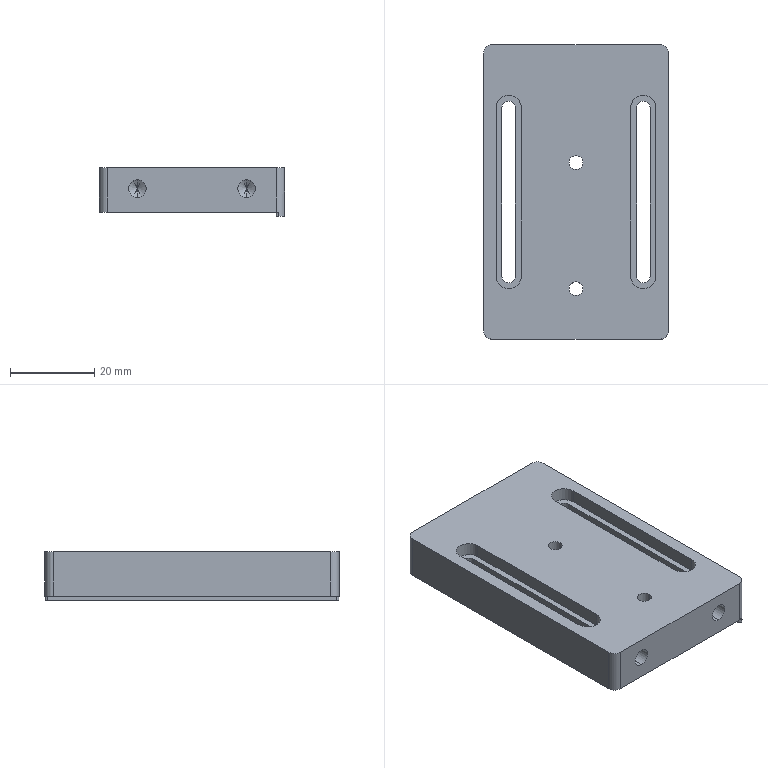Part | STEP file | Guide wheel mechanism revised.sldasm-Part-46 | 1 solid | 52 faces | box 44 x 70 x 11.6 mm | volume 26804 mm3 | cylinder 26 | plane 22 | cone 4 | commonest cylinder face diameters 2 x4 3.2 x4 3.3 x4 4 x4 4.2 x4 6 x4